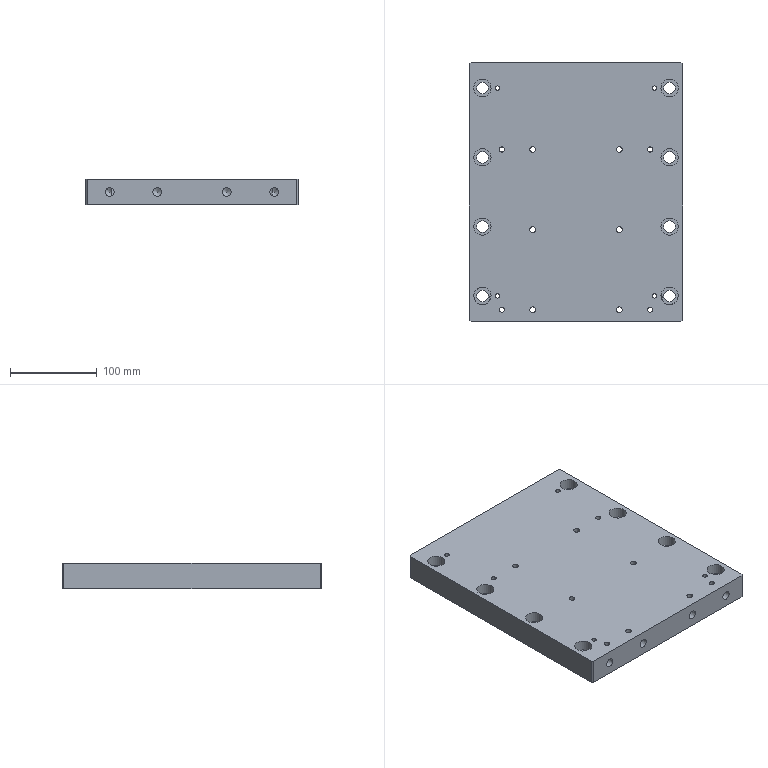CAM job | NX | 3-axis milling, drilling | part box 246 x 300 x 30 mm | stock box 246 x 300 x 30 mm
Tools:
number,name,description,diameter,corner_radius,flute_length,length,flutes
9,D10,平底铣刀-粗,10.0,0.0,35.0,75.0,2
10,D10-J,平底铣刀-精,10.0,0.0,35.0,75.0,2
2,D6倒角刀,倒角刀,6.0,0.0,3.0,25.0,2
23,D5铰刀,Drilling Tool,5.0,0.0,75.0,100.0,6
24,D6铰刀,Drilling Tool,6.0,0.0,75.0,100.0,6
1,C6定点钻,倒角刀,6.0,0.0,3.0,3.0,2
16,ZT6.8,钻头,6.8,0.0,35.0,50.0,2
19,ZT13.5,钻头,13.5,0.0,35.0,50.0,2
17,ZT4.9,Drilling Tool,4.9,0.0,35.0,50.0,2
18,ZT5.9,Drilling Tool,5.9,0.0,35.0,50.0,2
Operations:
program,operation,operation_type,tool,method,geometry_group,spindle_rpm,surface_speed,feed_per_tooth,feed_cut,feed_plunge,cut_length_mm,path_length_mm,cut_time_min,machine_time_min
B,等高往复层切开粗-中_COPY_COPY,ZLevelMilling,D10,分层开粗-切深K-步距G,W-B,3000.0,94.248,0.3333,2000.0,100.0,3391.287,4488.185,1.696,1.805
B,铣倒角_5,PlanarMilling,D6倒角刀,METHOD,W-B,4000.0,75.398,0.075,600.0,100.0,43.871,815.052,0.0731,0.1502
B,铣倒角_6,PlanarMilling,D6倒角刀,METHOD,W-B,4000.0,75.398,0.075,600.0,100.0,72.081,769.28,0.1201,0.1899
B,铣倒角_7,PlanarMilling,D6倒角刀,METHOD,W-B,4000.0,75.398,0.0375,300.0,100.0,143.492,866.737,0.4783,0.5506
B,C0.3封闭铣廓倒角6X45L_COPY_1,PlanarMilling,D6倒角刀,爬面_倒角-切深0-步距G,W-B,4000.0,75.398,0.125,1000.0,100.0,1509.514,2573.085,1.51,1.616
B,等高精光-中_COPY_COPY,ZLevelMilling,D10-J,侧刃精光-切深K-步距G,W-B,3000.0,94.248,0.1667,1000.0,100.0,38.376,1024.481,0.0384,0.137
A,等高往复层切开粗-中_COPY,ZLevelMilling,D10,分层开粗-切深K-步距G,W-A,3000.0,94.248,0.3333,2000.0,100.0,3391.287,4488.185,1.696,1.805
A,打点-深0.8,Operation,C6定点钻,NONE,W-A,3000.0,56.0,0.01,60.0,90.0,39.6,1155.733,0.66,0.7716
A,通孔-精孔6.0预钻,Operation,ZT4.9,NONE,W-A,1000.0,15.394,0.03,60.0,90.0,141.658,928.324,2.361,2.44
A,通孔-精孔6.0预钻_2,Operation,ZT5.9,NONE,W-A,1000.0,18.535,0.04,80.0,90.0,142.813,855.634,1.785,1.856
A,通孔-M8螺纹底孔,Operation,ZT6.8,NONE,W-A,600.0,12.818,0.1,120.0,90.0,231.258,977.542,1.927,2.002
A,沉头孔-钻孔0段,Operation,ZT13.5,NONE,W-A,500.0,21.206,0.12,120.0,90.0,296.447,1335.933,2.47,2.574
A,铣孔开粗D8_1,CylinderMilling,D10,NONE,W-A,4000.0,100.531,0.25,2000.0,100.0,13276.042,14388.842,6.638,6.749
A,铣孔精光D8_1,CylinderMilling,D10-J,精光步距切深关,W-A,4000.0,100.531,0.1,800.0,100.0,1031.154,2143.954,1.289,1.4
A,铣倒角_1,PlanarMilling,D6倒角刀,METHOD,W-A,4000.0,75.398,0.05,400.0,100.0,73.926,838.371,0.1848,0.2613
A,铣倒角_2,PlanarMilling,D6倒角刀,METHOD,W-A,4000.0,75.398,0.05,400.0,100.0,83.855,772.591,0.2096,0.2785
A,铣倒角_3,PlanarMilling,D6倒角刀,METHOD,W-A,4000.0,75.398,0.0625,500.0,100.0,140.862,862.907,0.2817,0.3539
A,铣倒角_4,PlanarMilling,D6倒角刀,NONE,W-A,4000.0,75.398,0.1,800.0,100.0,573.336,1553.753,0.7167,0.8147
A,C0.3封闭铣廓倒角6X45L_COPY,PlanarMilling,D6倒角刀,爬面_倒角-切深0-步距G,W-A,4000.0,75.398,0.125,1000.0,100.0,1107.604,1143.904,1.108,1.111
A,REAMING,Operation,D5铰刀,METHOD,W-A,500.0,7.854,0.0167,50.0,0.0,128.0,901.008,2.56,2.637
A,REAMING_2,Operation,D6铰刀,METHOD,W-A,500.0,9.425,0.0167,50.0,0.0,128.0,826.009,2.56,2.63
A,等高精光-中_COPY,ZLevelMilling,D10-J,侧刃精光-切深K-步距G,W-A,3000.0,94.248,0.1667,1000.0,100.0,38.376,999.642,0.0384,0.1345